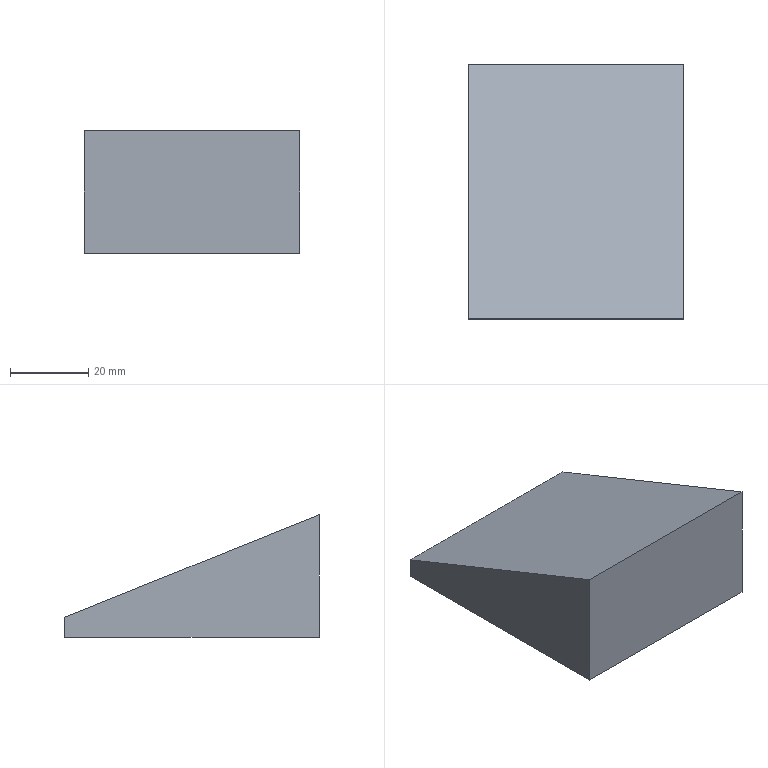Part | NX | features solid 2 | 1 solid | 6 faces | box 55 x 65 x 31.395 mm | volume 65293 mm3 | plane 6
STEP:
#1=CARTESIAN_POINT('',(-700.,525.,-104.867));
#2=VERTEX_POINT('',#1);
#3=CARTESIAN_POINT('',(-700.,460.,-78.605));
#4=VERTEX_POINT('',#3);
#5=CARTESIAN_POINT('',(-700.,-382.33,261.718));
#6=DIRECTION('',(0.,-0.9272,0.3746));
#7=VECTOR('',#6,1000.);
#8=LINE('',#5,#7);
#9=EDGE_CURVE('',#2,#4,#8,.T.);
#10=ORIENTED_EDGE('',*,*,#9,.F.);
#11=CARTESIAN_POINT('',(-700.,525.,-110.));
#12=VERTEX_POINT('',#11);
#13=CARTESIAN_POINT('',(-700.,525.,-68.));
#14=DIRECTION('',(0.,0.,-1.));
#15=VECTOR('',#14,1000.);
#16=LINE('',#13,#15);
#17=EDGE_CURVE('',#2,#12,#16,.T.);
#18=ORIENTED_EDGE('',*,*,#17,.T.);
#19=CARTESIAN_POINT('',(-700.,460.,-110.));
#20=VERTEX_POINT('',#19);
#21=CARTESIAN_POINT('',(-700.,-515.545,-110.));
#22=DIRECTION('',(0.,1.,0.));
#23=VECTOR('',#22,1000.);
#24=LINE('',#21,#23);
#25=EDGE_CURVE('',#20,#12,#24,.T.);
#26=ORIENTED_EDGE('',*,*,#25,.F.);
#27=CARTESIAN_POINT('',(-700.,460.,-68.));
#28=DIRECTION('',(0.,0.,-1.));
#29=VECTOR('',#28,1000.);
#30=LINE('',#27,#29);
#31=EDGE_CURVE('',#4,#20,#30,.T.);
#32=ORIENTED_EDGE('',*,*,#31,.F.);
#33=EDGE_LOOP('',(#10,#18,#26,#32));
#34=FACE_BOUND('',#33,.T.);
#35=CARTESIAN_POINT('',(-700.,-515.545,-68.));
#36=DIRECTION('',(-1.,0.,0.));
#37=DIRECTION('',(0.,0.,1.));
#38=AXIS2_PLACEMENT_3D('',#35,#36,#37);
#39=PLANE('',#38);
#40=ADVANCED_FACE('',(#34),#39,.T.);
#41=CARTESIAN_POINT('',(-645.,460.,-78.605));
#42=VERTEX_POINT('',#41);
#43=CARTESIAN_POINT('',(-645.,460.,-110.));
#44=VERTEX_POINT('',#43);
#45=CARTESIAN_POINT('',(-645.,460.,-68.));
#46=DIRECTION('',(0.,0.,-1.));
#47=VECTOR('',#46,1000.);
#48=LINE('',#45,#47);
#49=EDGE_CURVE('',#42,#44,#48,.T.);
#50=ORIENTED_EDGE('',*,*,#49,.F.);
#51=CARTESIAN_POINT('',(-2444.088,460.,-78.605));
#52=DIRECTION('',(-1.,0.,0.));
#53=VECTOR('',#52,1000.);
#54=LINE('',#51,#53);
#55=EDGE_CURVE('',#42,#4,#54,.T.);
#56=ORIENTED_EDGE('',*,*,#55,.T.);
#57=ORIENTED_EDGE('',*,*,#31,.T.);
#58=CARTESIAN_POINT('',(-2444.088,460.,-110.));
#59=DIRECTION('',(1.,0.,0.));
#60=VECTOR('',#59,1000.);
#61=LINE('',#58,#60);
#62=EDGE_CURVE('',#20,#44,#61,.T.);
#63=ORIENTED_EDGE('',*,*,#62,.T.);
#64=EDGE_LOOP('',(#50,#56,#57,#63));
#65=FACE_BOUND('',#64,.T.);
#66=CARTESIAN_POINT('',(-2444.088,460.,-68.));
#67=DIRECTION('',(0.,1.,0.));
#68=DIRECTION('',(0.,0.,1.));
#69=AXIS2_PLACEMENT_3D('',#66,#67,#68);
#70=PLANE('',#69);
#71=ADVANCED_FACE('',(#65),#70,.F.);
#72=CARTESIAN_POINT('',(-645.,525.,-104.867));
#73=VERTEX_POINT('',#72);
#74=CARTESIAN_POINT('',(-645.,525.,-110.));
#75=VERTEX_POINT('',#74);
#76=CARTESIAN_POINT('',(-645.,525.,-68.));
#77=DIRECTION('',(0.,0.,-1.));
#78=VECTOR('',#77,1000.);
#79=LINE('',#76,#78);
#80=EDGE_CURVE('',#73,#75,#79,.T.);
#81=ORIENTED_EDGE('',*,*,#80,.F.);
#82=CARTESIAN_POINT('',(-645.,-382.33,261.718));
#83=DIRECTION('',(0.,-0.9272,0.3746));
#84=VECTOR('',#83,1000.);
#85=LINE('',#82,#84);
#86=EDGE_CURVE('',#73,#42,#85,.T.);
#87=ORIENTED_EDGE('',*,*,#86,.T.);
#88=ORIENTED_EDGE('',*,*,#49,.T.);
#89=CARTESIAN_POINT('',(-645.,-515.545,-110.));
#90=DIRECTION('',(0.,1.,0.));
#91=VECTOR('',#90,1000.);
#92=LINE('',#89,#91);
#93=EDGE_CURVE('',#44,#75,#92,.T.);
#94=ORIENTED_EDGE('',*,*,#93,.T.);
#95=EDGE_LOOP('',(#81,#87,#88,#94));
#96=FACE_BOUND('',#95,.T.);
#97=CARTESIAN_POINT('',(-645.,-515.545,-68.));
#98=DIRECTION('',(-1.,0.,0.));
#99=DIRECTION('',(0.,0.,1.));
#100=AXIS2_PLACEMENT_3D('',#97,#98,#99);
#101=PLANE('',#100);
#102=ADVANCED_FACE('',(#96),#101,.F.);
#103=CARTESIAN_POINT('',(-2444.088,525.,-104.867));
#104=DIRECTION('',(-1.,0.,0.));
#105=VECTOR('',#104,1000.);
#106=LINE('',#103,#105);
#107=EDGE_CURVE('',#73,#2,#106,.T.);
#108=ORIENTED_EDGE('',*,*,#107,.F.);
#109=ORIENTED_EDGE('',*,*,#80,.T.);
#110=CARTESIAN_POINT('',(-2444.088,525.,-110.));
#111=DIRECTION('',(1.,0.,0.));
#112=VECTOR('',#111,1000.);
#113=LINE('',#110,#112);
#114=EDGE_CURVE('',#12,#75,#113,.T.);
#115=ORIENTED_EDGE('',*,*,#114,.F.);
#116=ORIENTED_EDGE('',*,*,#17,.F.);
#117=EDGE_LOOP('',(#108,#109,#115,#116));
#118=FACE_BOUND('',#117,.T.);
#119=CARTESIAN_POINT('',(-2444.088,525.,-68.));
#120=DIRECTION('',(0.,1.,0.));
#121=DIRECTION('',(0.,0.,1.));
#122=AXIS2_PLACEMENT_3D('',#119,#120,#121);
#123=PLANE('',#122);
#124=ADVANCED_FACE('',(#118),#123,.T.);
#125=ORIENTED_EDGE('',*,*,#25,.T.);
#126=ORIENTED_EDGE('',*,*,#114,.T.);
#127=ORIENTED_EDGE('',*,*,#93,.F.);
#128=ORIENTED_EDGE('',*,*,#62,.F.);
#129=EDGE_LOOP('',(#125,#126,#127,#128));
#130=FACE_BOUND('',#129,.T.);
#131=CARTESIAN_POINT('',(-489.801,305.407,-110.));
#132=DIRECTION('',(0.,0.,1.));
#133=DIRECTION('',(1.,0.,0.));
#134=AXIS2_PLACEMENT_3D('',#131,#132,#133);
#135=PLANE('',#134);
#136=ADVANCED_FACE('',(#130),#135,.F.);
#137=ORIENTED_EDGE('',*,*,#107,.T.);
#138=ORIENTED_EDGE('',*,*,#9,.T.);
#139=ORIENTED_EDGE('',*,*,#55,.F.);
#140=ORIENTED_EDGE('',*,*,#86,.F.);
#141=EDGE_LOOP('',(#137,#138,#139,#140));
#142=FACE_BOUND('',#141,.T.);
#143=CARTESIAN_POINT('',(-646.881,458.254,-77.9));
#144=DIRECTION('',(0.,-0.3746,-0.9272));
#145=DIRECTION('',(0.,0.9272,-0.3746));
#146=AXIS2_PLACEMENT_3D('',#143,#144,#145);
#147=PLANE('',#146);
#148=ADVANCED_FACE('',(#142),#147,.F.);
#149=CLOSED_SHELL('',(#40,#71,#102,#124,#136,#148));
#150=MANIFOLD_SOLID_BREP('',#149);
#151=(LENGTH_UNIT()NAMED_UNIT(*)SI_UNIT(.MILLI.,.METRE.));
#152=UNCERTAINTY_MEASURE_WITH_UNIT(LENGTH_MEASURE(0.00001),#151,'','');
#153=(NAMED_UNIT(*)PLANE_ANGLE_UNIT()SI_UNIT($,.RADIAN.));
#154=(NAMED_UNIT(*)SI_UNIT($,.STERADIAN.)SOLID_ANGLE_UNIT());
#155=(GEOMETRIC_REPRESENTATION_CONTEXT(3)GLOBAL_UNCERTAINTY_ASSIGNED_CONTEXT((#152))GLOBAL_UNIT_ASSIGNED_CONTEXT((#151,#153,#154))REPRESENTATION_CONTEXT('',''));
#156=ADVANCED_BREP_SHAPE_REPRESENTATION('',(#150),#155);